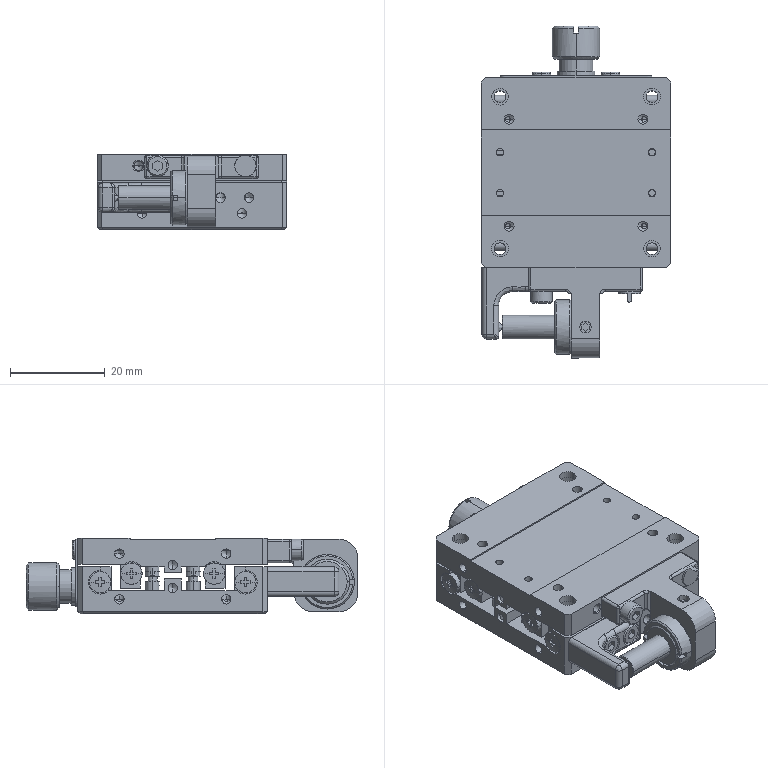Part | SolidWorks | 26 solids | 1155 faces | box 40 x 69.9 x 16 mm | volume 24184 mm3 | cylinder 435 | plane 409 | cone 229 | spline 46 | torus 36 | commonest cylinder face diameters 2.1 x89 2 x61 2.013 x58 3 x28 1.567 x24 4.5 x24